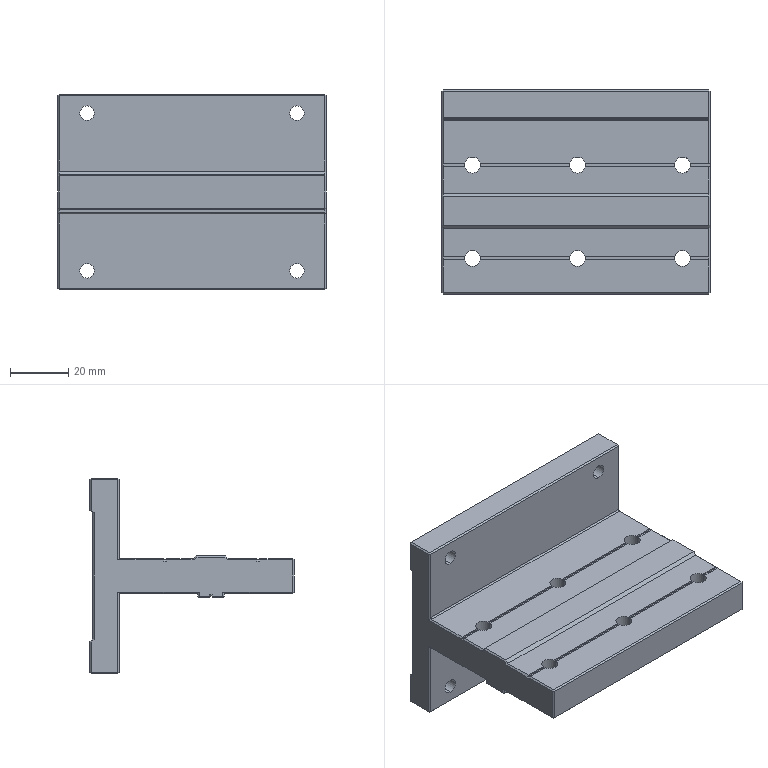Part | SolidWorks | features MBimport 1 | 1 solid | 145 faces | box 92 x 70 x 67 mm | volume 123331 mm3 | plane 121 | cylinder 24 | commonest cylinder face diameters 5.5 x12 5 x8 1 x4